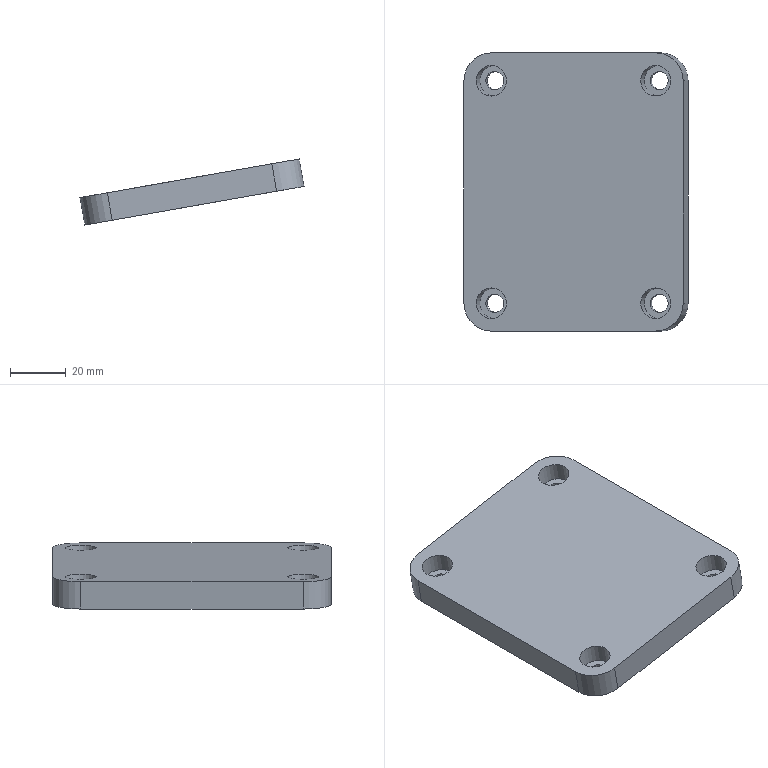Part | STEP file | solid 178 | 1 solid | 22 faces | box 80.521 x 100 x 23.74 mm | volume 76082 mm3 | cylinder 12 | plane 10 | commonest cylinder face diameters 6.5 x4 11 x4 20 x4